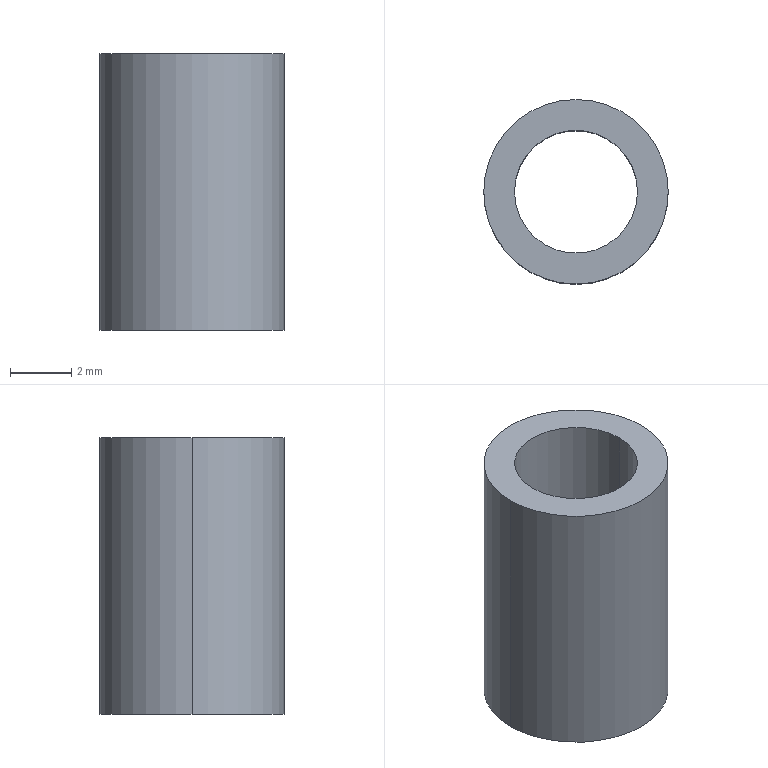Part | NX | features BREP 1 | 1 solid | 6 faces | box 6 x 6 x 9 mm | volume 141.372 mm3 | cylinder 4 | plane 2 | commonest cylinder face diameters 4 x2 6 x2
STEP:
#1=CARTESIAN_POINT('',(-3.,0.,-4.5));
#2=VERTEX_POINT('',#1);
#3=CARTESIAN_POINT('',(3.,0.,-4.5));
#4=VERTEX_POINT('',#3);
#5=CARTESIAN_POINT('',(0.,0.,-4.5));
#6=DIRECTION('',(0.,0.,1.));
#7=DIRECTION('',(1.,0.,0.));
#8=AXIS2_PLACEMENT_3D('',#5,#6,#7);
#9=CIRCLE('',#8,3.);
#10=EDGE_CURVE('',#2,#4,#9,.T.);
#11=ORIENTED_EDGE('',*,*,#10,.F.);
#12=CARTESIAN_POINT('',(0.,0.,-4.5));
#13=DIRECTION('',(0.,0.,1.));
#14=DIRECTION('',(1.,0.,0.));
#15=AXIS2_PLACEMENT_3D('',#12,#13,#14);
#16=CIRCLE('',#15,3.);
#17=EDGE_CURVE('',#4,#2,#16,.T.);
#18=ORIENTED_EDGE('',*,*,#17,.F.);
#19=EDGE_LOOP('',(#11,#18));
#20=FACE_BOUND('',#19,.T.);
#21=CARTESIAN_POINT('',(-2.,0.,-4.5));
#22=VERTEX_POINT('',#21);
#23=CARTESIAN_POINT('',(2.,0.,-4.5));
#24=VERTEX_POINT('',#23);
#25=CARTESIAN_POINT('',(0.,0.,-4.5));
#26=DIRECTION('',(0.,0.,1.));
#27=DIRECTION('',(1.,0.,0.));
#28=AXIS2_PLACEMENT_3D('',#25,#26,#27);
#29=CIRCLE('',#28,2.);
#30=EDGE_CURVE('',#22,#24,#29,.T.);
#31=ORIENTED_EDGE('',*,*,#30,.T.);
#32=CARTESIAN_POINT('',(0.,0.,-4.5));
#33=DIRECTION('',(0.,0.,1.));
#34=DIRECTION('',(1.,0.,0.));
#35=AXIS2_PLACEMENT_3D('',#32,#33,#34);
#36=CIRCLE('',#35,2.);
#37=EDGE_CURVE('',#24,#22,#36,.T.);
#38=ORIENTED_EDGE('',*,*,#37,.T.);
#39=EDGE_LOOP('',(#31,#38));
#40=FACE_BOUND('',#39,.T.);
#41=CARTESIAN_POINT('',(0.,0.,-4.5));
#42=DIRECTION('',(0.,0.,1.));
#43=DIRECTION('',(1.,0.,0.));
#44=AXIS2_PLACEMENT_3D('',#41,#42,#43);
#45=PLANE('',#44);
#46=ADVANCED_FACE('',(#20,#40),#45,.F.);
#47=CARTESIAN_POINT('',(-3.,0.,4.5));
#48=VERTEX_POINT('',#47);
#49=CARTESIAN_POINT('',(3.,0.,4.5));
#50=VERTEX_POINT('',#49);
#51=CARTESIAN_POINT('',(0.,0.,4.5));
#52=DIRECTION('',(0.,0.,1.));
#53=DIRECTION('',(1.,0.,0.));
#54=AXIS2_PLACEMENT_3D('',#51,#52,#53);
#55=CIRCLE('',#54,3.);
#56=EDGE_CURVE('',#48,#50,#55,.T.);
#57=ORIENTED_EDGE('',*,*,#56,.T.);
#58=CARTESIAN_POINT('',(0.,0.,4.5));
#59=DIRECTION('',(0.,0.,1.));
#60=DIRECTION('',(1.,0.,0.));
#61=AXIS2_PLACEMENT_3D('',#58,#59,#60);
#62=CIRCLE('',#61,3.);
#63=EDGE_CURVE('',#50,#48,#62,.T.);
#64=ORIENTED_EDGE('',*,*,#63,.T.);
#65=EDGE_LOOP('',(#57,#64));
#66=FACE_BOUND('',#65,.T.);
#67=CARTESIAN_POINT('',(-2.,0.,4.5));
#68=VERTEX_POINT('',#67);
#69=CARTESIAN_POINT('',(2.,0.,4.5));
#70=VERTEX_POINT('',#69);
#71=CARTESIAN_POINT('',(0.,0.,4.5));
#72=DIRECTION('',(0.,0.,1.));
#73=DIRECTION('',(1.,0.,0.));
#74=AXIS2_PLACEMENT_3D('',#71,#72,#73);
#75=CIRCLE('',#74,2.);
#76=EDGE_CURVE('',#68,#70,#75,.T.);
#77=ORIENTED_EDGE('',*,*,#76,.F.);
#78=CARTESIAN_POINT('',(0.,0.,4.5));
#79=DIRECTION('',(0.,0.,1.));
#80=DIRECTION('',(1.,0.,0.));
#81=AXIS2_PLACEMENT_3D('',#78,#79,#80);
#82=CIRCLE('',#81,2.);
#83=EDGE_CURVE('',#70,#68,#82,.T.);
#84=ORIENTED_EDGE('',*,*,#83,.F.);
#85=EDGE_LOOP('',(#77,#84));
#86=FACE_BOUND('',#85,.T.);
#87=CARTESIAN_POINT('',(0.,0.,4.5));
#88=DIRECTION('',(0.,0.,1.));
#89=DIRECTION('',(1.,0.,0.));
#90=AXIS2_PLACEMENT_3D('',#87,#88,#89);
#91=PLANE('',#90);
#92=ADVANCED_FACE('',(#66,#86),#91,.T.);
#93=CARTESIAN_POINT('',(3.,0.,4.5));
#94=DIRECTION('',(0.,0.,-1.));
#95=VECTOR('',#94,1000.);
#96=LINE('',#93,#95);
#97=EDGE_CURVE('',#50,#4,#96,.T.);
#98=ORIENTED_EDGE('',*,*,#97,.F.);
#99=ORIENTED_EDGE('',*,*,#56,.F.);
#100=CARTESIAN_POINT('',(-3.,0.,4.5));
#101=DIRECTION('',(0.,0.,-1.));
#102=VECTOR('',#101,1000.);
#103=LINE('',#100,#102);
#104=EDGE_CURVE('',#48,#2,#103,.T.);
#105=ORIENTED_EDGE('',*,*,#104,.T.);
#106=ORIENTED_EDGE('',*,*,#10,.T.);
#107=EDGE_LOOP('',(#98,#99,#105,#106));
#108=FACE_BOUND('',#107,.T.);
#109=CARTESIAN_POINT('',(0.,0.,4.5));
#110=DIRECTION('',(0.,0.,-1.));
#111=DIRECTION('',(-1.,0.,0.));
#112=AXIS2_PLACEMENT_3D('',#109,#110,#111);
#113=CYLINDRICAL_SURFACE('',#112,3.);
#114=ADVANCED_FACE('',(#108),#113,.T.);
#115=CARTESIAN_POINT('',(2.,0.,4.5));
#116=DIRECTION('',(0.,0.,-1.));
#117=VECTOR('',#116,1000.);
#118=LINE('',#115,#117);
#119=EDGE_CURVE('',#70,#24,#118,.T.);
#120=ORIENTED_EDGE('',*,*,#119,.F.);
#121=ORIENTED_EDGE('',*,*,#83,.T.);
#122=CARTESIAN_POINT('',(-2.,0.,4.5));
#123=DIRECTION('',(0.,0.,-1.));
#124=VECTOR('',#123,1000.);
#125=LINE('',#122,#124);
#126=EDGE_CURVE('',#68,#22,#125,.T.);
#127=ORIENTED_EDGE('',*,*,#126,.T.);
#128=ORIENTED_EDGE('',*,*,#37,.F.);
#129=EDGE_LOOP('',(#120,#121,#127,#128));
#130=FACE_BOUND('',#129,.T.);
#131=CARTESIAN_POINT('',(0.,0.,4.5));
#132=DIRECTION('',(0.,0.,-1.));
#133=DIRECTION('',(-1.,0.,0.));
#134=AXIS2_PLACEMENT_3D('',#131,#132,#133);
#135=CYLINDRICAL_SURFACE('',#134,2.);
#136=ADVANCED_FACE('',(#130),#135,.F.);
#137=ORIENTED_EDGE('',*,*,#76,.T.);
#138=ORIENTED_EDGE('',*,*,#119,.T.);
#139=ORIENTED_EDGE('',*,*,#30,.F.);
#140=ORIENTED_EDGE('',*,*,#126,.F.);
#141=EDGE_LOOP('',(#137,#138,#139,#140));
#142=FACE_BOUND('',#141,.T.);
#143=CARTESIAN_POINT('',(0.,0.,4.5));
#144=DIRECTION('',(0.,0.,-1.));
#145=DIRECTION('',(-1.,0.,0.));
#146=AXIS2_PLACEMENT_3D('',#143,#144,#145);
#147=CYLINDRICAL_SURFACE('',#146,2.);
#148=ADVANCED_FACE('',(#142),#147,.F.);
#149=ORIENTED_EDGE('',*,*,#63,.F.);
#150=ORIENTED_EDGE('',*,*,#97,.T.);
#151=ORIENTED_EDGE('',*,*,#17,.T.);
#152=ORIENTED_EDGE('',*,*,#104,.F.);
#153=EDGE_LOOP('',(#149,#150,#151,#152));
#154=FACE_BOUND('',#153,.T.);
#155=CARTESIAN_POINT('',(0.,0.,4.5));
#156=DIRECTION('',(0.,0.,-1.));
#157=DIRECTION('',(-1.,0.,0.));
#158=AXIS2_PLACEMENT_3D('',#155,#156,#157);
#159=CYLINDRICAL_SURFACE('',#158,3.);
#160=ADVANCED_FACE('',(#154),#159,.T.);
#161=CLOSED_SHELL('',(#46,#92,#114,#136,#148,#160));
#162=MANIFOLD_SOLID_BREP('',#161);
#163=(LENGTH_UNIT()NAMED_UNIT(*)SI_UNIT(.MILLI.,.METRE.));
#164=UNCERTAINTY_MEASURE_WITH_UNIT(LENGTH_MEASURE(0.00001),#163,'','');
#165=(NAMED_UNIT(*)PLANE_ANGLE_UNIT()SI_UNIT($,.RADIAN.));
#166=(NAMED_UNIT(*)SI_UNIT($,.STERADIAN.)SOLID_ANGLE_UNIT());
#167=(GEOMETRIC_REPRESENTATION_CONTEXT(3)GLOBAL_UNCERTAINTY_ASSIGNED_CONTEXT((#164))GLOBAL_UNIT_ASSIGNED_CONTEXT((#163,#165,#166))REPRESENTATION_CONTEXT('',''));
#168=ADVANCED_BREP_SHAPE_REPRESENTATION('',(#162),#167);